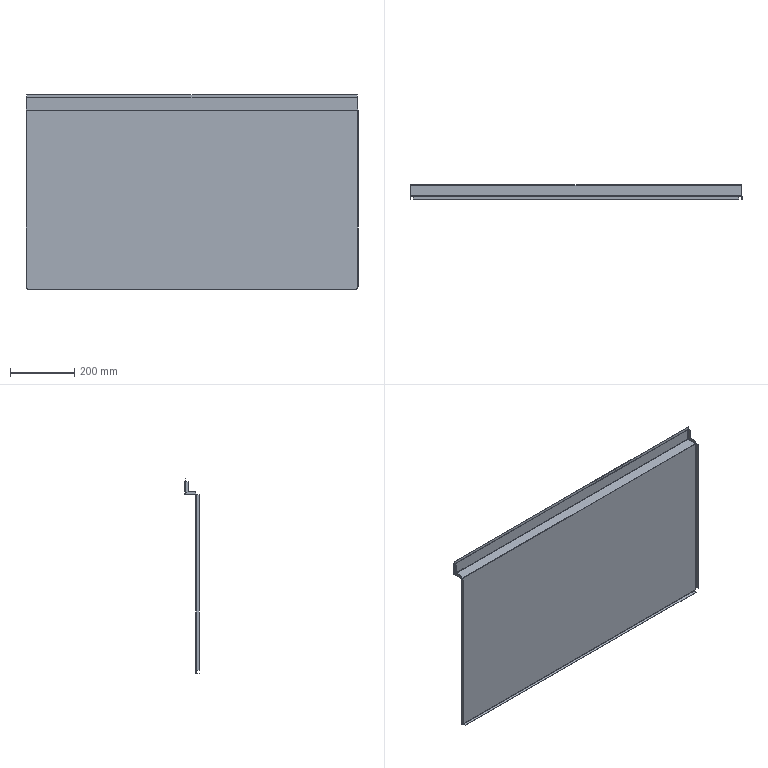Part | SolidWorks | features EdgeFlange 5, Fillet 1, FlatPattern 1, SMBaseFlange 1, SheetMetal 1 | 1 solid | 105 faces | box 1037 x 44.4 x 608.8 mm | volume 412914 mm3 | plane 78 | cylinder 23 | spline 4 | commonest cylinder face diameters 1 x9 2.2 x9 20 x2 0.2 x1 1.2 x1 1.4 x1